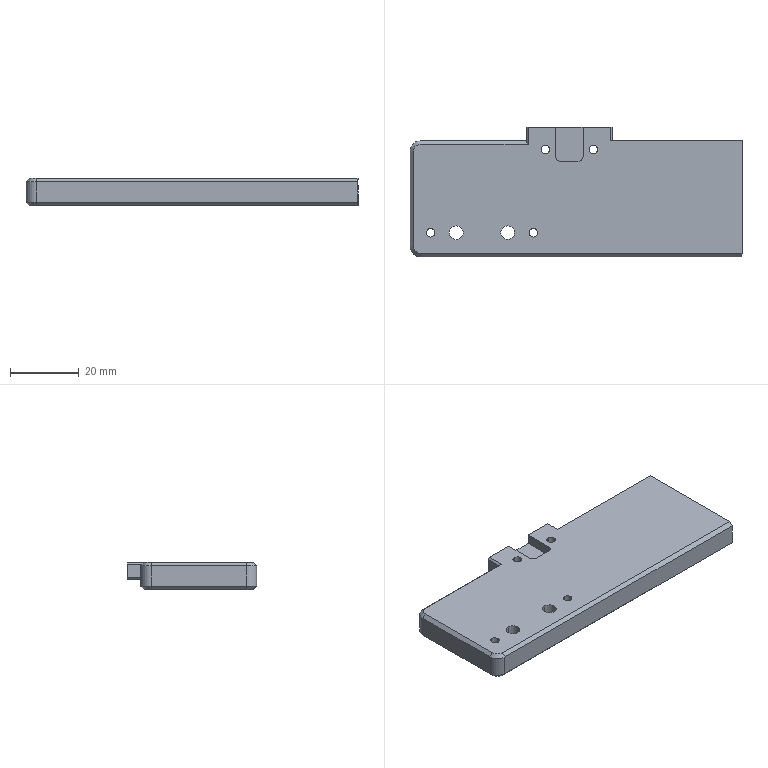Part | 1 solid | 74 faces | box 96.9 x 37.8 x 8 mm | volume 25239 mm3 | cylinder 30 | plane 30 | cone 14 | commonest cylinder face diameters 2.5 x8 4 x8 3.3 x6 5 x4 3 x2 6 x2